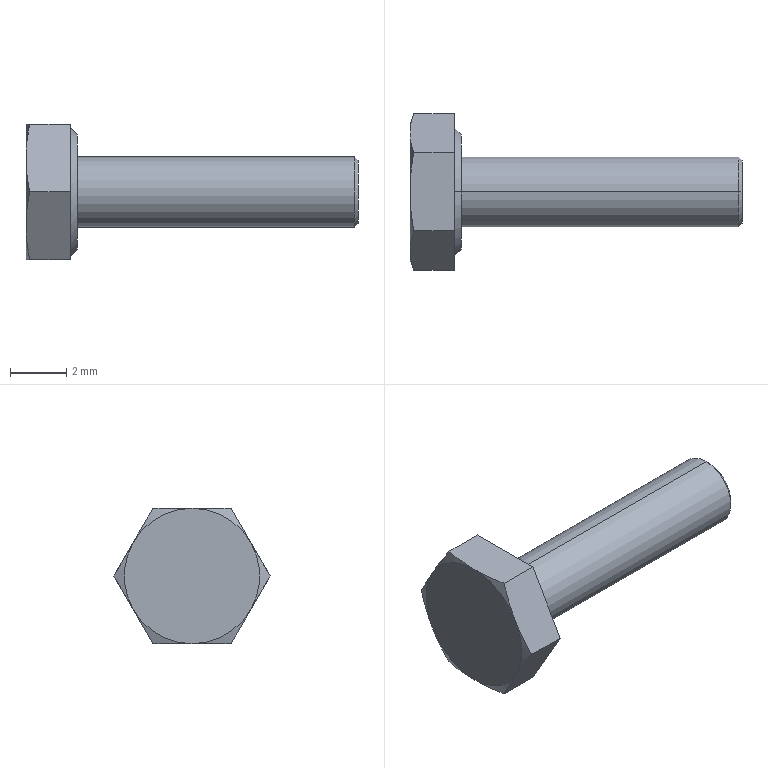Part | SolidWorks | features RevCut 3, Boss 1, Chamfer 1, Extrusion 1, Fillet 1, LPattern 1 | 1 solid | 22 faces | box 11.825 x 5.566 x 4.82 mm | volume 84.307 mm3 | cone 10 | plane 10 | cylinder 2 | commonest cylinder face diameters 2.5 x2
STEP:
#1=CARTESIAN_POINT('',(11.825,0.,-1.125));
#2=VERTEX_POINT('',#1);
#3=CARTESIAN_POINT('',(11.825,0.,1.125));
#4=VERTEX_POINT('',#3);
#5=CARTESIAN_POINT('',(11.825,0.,0.));
#6=DIRECTION('',(1.,0.,0.));
#7=DIRECTION('',(0.,0.,-1.));
#8=AXIS2_PLACEMENT_3D('',#5,#6,#7);
#9=CIRCLE('',#8,1.125);
#10=EDGE_CURVE('',#2,#4,#9,.T.);
#11=ORIENTED_EDGE('',*,*,#10,.F.);
#12=CARTESIAN_POINT('',(11.7,0.,-1.25));
#13=VERTEX_POINT('',#12);
#14=CARTESIAN_POINT('',(11.825,0.,-1.125));
#15=DIRECTION('',(-0.7071,0.,-0.7071));
#16=VECTOR('',#15,1000.);
#17=LINE('',#14,#16);
#18=EDGE_CURVE('',#2,#13,#17,.T.);
#19=ORIENTED_EDGE('',*,*,#18,.T.);
#20=CARTESIAN_POINT('',(11.7,0.,1.25));
#21=VERTEX_POINT('',#20);
#22=CARTESIAN_POINT('',(11.7,0.,0.));
#23=DIRECTION('',(-1.,0.,0.));
#24=DIRECTION('',(0.,0.,-1.));
#25=AXIS2_PLACEMENT_3D('',#22,#23,#24);
#26=CIRCLE('',#25,1.25);
#27=EDGE_CURVE('',#21,#13,#26,.T.);
#28=ORIENTED_EDGE('',*,*,#27,.F.);
#29=CARTESIAN_POINT('',(11.825,0.,1.125));
#30=DIRECTION('',(-0.7071,0.,0.7071));
#31=VECTOR('',#30,1000.);
#32=LINE('',#29,#31);
#33=EDGE_CURVE('',#4,#21,#32,.T.);
#34=ORIENTED_EDGE('',*,*,#33,.F.);
#35=EDGE_LOOP('',(#11,#19,#28,#34));
#36=FACE_OUTER_BOUND('',#35,.T.);
#37=CARTESIAN_POINT('',(11.825,0.,0.));
#38=DIRECTION('',(-1.,0.,0.));
#39=DIRECTION('',(0.,0.,1.));
#40=AXIS2_PLACEMENT_3D('',#37,#38,#39);
#41=CONICAL_SURFACE('',#40,1.125,0.7854);
#42=ADVANCED_FACE('',(#36),#41,.T.);
#43=ORIENTED_EDGE('',*,*,#27,.T.);
#44=CARTESIAN_POINT('',(1.825,0.,-1.25));
#45=VERTEX_POINT('',#44);
#46=CARTESIAN_POINT('',(11.825,0.,-1.25));
#47=DIRECTION('',(-1.,0.,0.));
#48=VECTOR('',#47,1000.);
#49=LINE('',#46,#48);
#50=EDGE_CURVE('',#13,#45,#49,.T.);
#51=ORIENTED_EDGE('',*,*,#50,.T.);
#52=CARTESIAN_POINT('',(1.825,0.,1.25));
#53=VERTEX_POINT('',#52);
#54=CARTESIAN_POINT('',(1.825,0.,0.));
#55=DIRECTION('',(1.,0.,0.));
#56=DIRECTION('',(0.,0.,-1.));
#57=AXIS2_PLACEMENT_3D('',#54,#55,#56);
#58=CIRCLE('',#57,1.25);
#59=EDGE_CURVE('',#45,#53,#58,.T.);
#60=ORIENTED_EDGE('',*,*,#59,.T.);
#61=CARTESIAN_POINT('',(11.825,0.,1.25));
#62=DIRECTION('',(-1.,0.,0.));
#63=VECTOR('',#62,1000.);
#64=LINE('',#61,#63);
#65=EDGE_CURVE('',#21,#53,#64,.T.);
#66=ORIENTED_EDGE('',*,*,#65,.F.);
#67=EDGE_LOOP('',(#43,#51,#60,#66));
#68=FACE_OUTER_BOUND('',#67,.T.);
#69=CARTESIAN_POINT('',(11.825,0.,0.));
#70=DIRECTION('',(-1.,0.,0.));
#71=DIRECTION('',(0.,0.,1.));
#72=AXIS2_PLACEMENT_3D('',#69,#70,#71);
#73=CYLINDRICAL_SURFACE('',#72,1.25);
#74=ADVANCED_FACE('',(#68),#73,.T.);
#75=CARTESIAN_POINT('',(1.825,0.,2.035));
#76=VERTEX_POINT('',#75);
#77=CARTESIAN_POINT('',(1.825,0.,-2.035));
#78=VERTEX_POINT('',#77);
#79=CARTESIAN_POINT('',(1.825,0.,0.));
#80=DIRECTION('',(-1.,0.,0.));
#81=DIRECTION('',(0.,0.,1.));
#82=AXIS2_PLACEMENT_3D('',#79,#80,#81);
#83=CIRCLE('',#82,2.035);
#84=EDGE_CURVE('',#76,#78,#83,.T.);
#85=ORIENTED_EDGE('',*,*,#84,.T.);
#86=CARTESIAN_POINT('',(1.575,0.,-2.285));
#87=VERTEX_POINT('',#86);
#88=CARTESIAN_POINT('',(1.575,0.,-2.285));
#89=DIRECTION('',(-0.7071,0.,-0.7071));
#90=VECTOR('',#89,1000.);
#91=LINE('',#88,#90);
#92=EDGE_CURVE('',#78,#87,#91,.T.);
#93=ORIENTED_EDGE('',*,*,#92,.T.);
#94=CARTESIAN_POINT('',(1.575,0.,2.285));
#95=VERTEX_POINT('',#94);
#96=CARTESIAN_POINT('',(1.575,0.,0.));
#97=DIRECTION('',(-1.,0.,0.));
#98=DIRECTION('',(0.,0.,1.));
#99=AXIS2_PLACEMENT_3D('',#96,#97,#98);
#100=CIRCLE('',#99,2.285);
#101=EDGE_CURVE('',#95,#87,#100,.T.);
#102=ORIENTED_EDGE('',*,*,#101,.F.);
#103=CARTESIAN_POINT('',(1.575,0.,2.285));
#104=DIRECTION('',(-0.7071,0.,0.7071));
#105=VECTOR('',#104,1000.);
#106=LINE('',#103,#105);
#107=EDGE_CURVE('',#76,#95,#106,.T.);
#108=ORIENTED_EDGE('',*,*,#107,.F.);
#109=EDGE_LOOP('',(#85,#93,#102,#108));
#110=FACE_OUTER_BOUND('',#109,.T.);
#111=CARTESIAN_POINT('',(1.575,0.,0.));
#112=DIRECTION('',(-1.,0.,0.));
#113=DIRECTION('',(0.,0.,1.));
#114=AXIS2_PLACEMENT_3D('',#111,#112,#113);
#115=CONICAL_SURFACE('',#114,2.285,0.7854);
#116=ADVANCED_FACE('',(#110),#115,.T.);
#117=ORIENTED_EDGE('',*,*,#84,.F.);
#118=CARTESIAN_POINT('',(1.825,0.,0.));
#119=DIRECTION('',(-1.,0.,0.));
#120=DIRECTION('',(0.,0.,1.));
#121=AXIS2_PLACEMENT_3D('',#118,#119,#120);
#122=CIRCLE('',#121,2.035);
#123=EDGE_CURVE('',#78,#76,#122,.T.);
#124=ORIENTED_EDGE('',*,*,#123,.F.);
#125=EDGE_LOOP('',(#117,#124));
#126=FACE_OUTER_BOUND('',#125,.T.);
#127=CARTESIAN_POINT('',(1.825,0.,0.));
#128=DIRECTION('',(1.,0.,0.));
#129=DIRECTION('',(0.,0.,-1.));
#130=AXIS2_PLACEMENT_3D('',#127,#128,#129);
#131=CIRCLE('',#130,1.25);
#132=EDGE_CURVE('',#53,#45,#131,.T.);
#133=ORIENTED_EDGE('',*,*,#132,.F.);
#134=ORIENTED_EDGE('',*,*,#59,.F.);
#135=EDGE_LOOP('',(#133,#134));
#136=FACE_BOUND('',#135,.T.);
#137=CARTESIAN_POINT('',(1.825,-1.391,-2.41));
#138=DIRECTION('',(1.,0.,0.));
#139=DIRECTION('',(0.,0.,-1.));
#140=AXIS2_PLACEMENT_3D('',#137,#138,#139);
#141=PLANE('',#140);
#142=ADVANCED_FACE('',(#126,#136),#141,.T.);
#143=CARTESIAN_POINT('',(0.1357,-1.391,-2.41));
#144=VERTEX_POINT('',#143);
#145=CARTESIAN_POINT('',(0.,-2.087,-1.205));
#146=VERTEX_POINT('',#145);
#147=CARTESIAN_POINT('',(0.1357,-1.391,-2.41));
#148=CARTESIAN_POINT('',(0.05129,-1.623,-2.008));
#149=CARTESIAN_POINT('',(0.,-1.855,-1.607));
#150=CARTESIAN_POINT('',(0.,-2.087,-1.205));
#151=B_SPLINE_CURVE_WITH_KNOTS('',3,(#147,#148,#149,#150),.UNSPECIFIED.,.F.,.F.,(4,4),(0.000000231,0.001392),.UNSPECIFIED.);
#152=EDGE_CURVE('',#144,#146,#151,.T.);
#153=ORIENTED_EDGE('',*,*,#152,.F.);
#154=CARTESIAN_POINT('',(1.575,-1.391,-2.41));
#155=VERTEX_POINT('',#154);
#156=CARTESIAN_POINT('',(1.825,-1.391,-2.41));
#157=DIRECTION('',(-1.,0.,0.));
#158=VECTOR('',#157,1000.);
#159=LINE('',#156,#158);
#160=EDGE_CURVE('',#155,#144,#159,.T.);
#161=ORIENTED_EDGE('',*,*,#160,.F.);
#162=CARTESIAN_POINT('',(1.575,-2.783,0.));
#163=VERTEX_POINT('',#162);
#164=CARTESIAN_POINT('',(1.575,-2.783,0.));
#165=DIRECTION('',(0.,0.5,-0.866));
#166=VECTOR('',#165,1000.);
#167=LINE('',#164,#166);
#168=EDGE_CURVE('',#163,#155,#167,.T.);
#169=ORIENTED_EDGE('',*,*,#168,.F.);
#170=CARTESIAN_POINT('',(0.1357,-2.783,0.));
#171=VERTEX_POINT('',#170);
#172=CARTESIAN_POINT('',(1.825,-2.783,0.));
#173=DIRECTION('',(-1.,0.,0.));
#174=VECTOR('',#173,1000.);
#175=LINE('',#172,#174);
#176=EDGE_CURVE('',#163,#171,#175,.T.);
#177=ORIENTED_EDGE('',*,*,#176,.T.);
#178=CARTESIAN_POINT('',(0.,-2.087,-1.205));
#179=CARTESIAN_POINT('',(0.,-2.319,-0.8033));
#180=CARTESIAN_POINT('',(0.05129,-2.551,-0.4017));
#181=CARTESIAN_POINT('',(0.1357,-2.783,0.));
#182=B_SPLINE_CURVE_WITH_KNOTS('',3,(#178,#179,#180,#181),.UNSPECIFIED.,.F.,.F.,(4,4),(0.001392,0.002783),.UNSPECIFIED.);
#183=EDGE_CURVE('',#146,#171,#182,.T.);
#184=ORIENTED_EDGE('',*,*,#183,.F.);
#185=EDGE_LOOP('',(#153,#161,#169,#177,#184));
#186=FACE_OUTER_BOUND('',#185,.T.);
#187=CARTESIAN_POINT('',(1.825,-2.783,0.));
#188=DIRECTION('',(0.,0.866,0.5));
#189=DIRECTION('',(0.,-0.5,0.866));
#190=AXIS2_PLACEMENT_3D('',#187,#188,#189);
#191=PLANE('',#190);
#192=ADVANCED_FACE('',(#186),#191,.F.);
#193=CARTESIAN_POINT('',(0.1357,1.391,-2.41));
#194=VERTEX_POINT('',#193);
#195=CARTESIAN_POINT('',(0.,0.,-2.41));
#196=VERTEX_POINT('',#195);
#197=CARTESIAN_POINT('',(0.1357,1.391,-2.41));
#198=CARTESIAN_POINT('',(0.05152,0.9289,-2.41));
#199=CARTESIAN_POINT('',(0.,0.4648,-2.41));
#200=CARTESIAN_POINT('',(0.,0.,-2.41));
#201=B_SPLINE_CURVE_WITH_KNOTS('',3,(#197,#198,#199,#200),.UNSPECIFIED.,.F.,.F.,(4,4),(0.005017,0.00642),.UNSPECIFIED.);
#202=EDGE_CURVE('',#194,#196,#201,.T.);
#203=ORIENTED_EDGE('',*,*,#202,.F.);
#204=CARTESIAN_POINT('',(1.575,1.391,-2.41));
#205=VERTEX_POINT('',#204);
#206=CARTESIAN_POINT('',(1.825,1.391,-2.41));
#207=DIRECTION('',(-1.,0.,0.));
#208=VECTOR('',#207,1000.);
#209=LINE('',#206,#208);
#210=EDGE_CURVE('',#205,#194,#209,.T.);
#211=ORIENTED_EDGE('',*,*,#210,.F.);
#212=CARTESIAN_POINT('',(1.575,-1.391,-2.41));
#213=DIRECTION('',(0.,1.,0.));
#214=VECTOR('',#213,1000.);
#215=LINE('',#212,#214);
#216=EDGE_CURVE('',#155,#205,#215,.T.);
#217=ORIENTED_EDGE('',*,*,#216,.F.);
#218=ORIENTED_EDGE('',*,*,#160,.T.);
#219=CARTESIAN_POINT('',(0.,0.,-2.41));
#220=CARTESIAN_POINT('',(0.,-0.4634,-2.41));
#221=CARTESIAN_POINT('',(0.05185,-0.9307,-2.41));
#222=CARTESIAN_POINT('',(0.1357,-1.391,-2.41));
#223=B_SPLINE_CURVE_WITH_KNOTS('',3,(#219,#220,#221,#222),.UNSPECIFIED.,.F.,.F.,(4,4),(0.00642,0.007819),.UNSPECIFIED.);
#224=EDGE_CURVE('',#196,#144,#223,.T.);
#225=ORIENTED_EDGE('',*,*,#224,.F.);
#226=EDGE_LOOP('',(#203,#211,#217,#218,#225));
#227=FACE_OUTER_BOUND('',#226,.T.);
#228=CARTESIAN_POINT('',(1.825,-1.391,-2.41));
#229=DIRECTION('',(0.,0.,1.));
#230=DIRECTION('',(1.,0.,0.));
#231=AXIS2_PLACEMENT_3D('',#228,#229,#230);
#232=PLANE('',#231);
#233=ADVANCED_FACE('',(#227),#232,.F.);
#234=CARTESIAN_POINT('',(0.1357,2.783,0.));
#235=VERTEX_POINT('',#234);
#236=CARTESIAN_POINT('',(0.,2.087,-1.205));
#237=VERTEX_POINT('',#236);
#238=CARTESIAN_POINT('',(0.1357,2.783,0.));
#239=CARTESIAN_POINT('',(0.05129,2.551,-0.4017));
#240=CARTESIAN_POINT('',(0.,2.319,-0.8033));
#241=CARTESIAN_POINT('',(0.,2.087,-1.205));
#242=B_SPLINE_CURVE_WITH_KNOTS('',3,(#238,#239,#240,#241),.UNSPECIFIED.,.F.,.F.,(4,4),(0.000000231,0.001392),.UNSPECIFIED.);
#243=EDGE_CURVE('',#235,#237,#242,.T.);
#244=ORIENTED_EDGE('',*,*,#243,.F.);
#245=CARTESIAN_POINT('',(1.575,2.783,0.));
#246=VERTEX_POINT('',#245);
#247=CARTESIAN_POINT('',(1.825,2.783,0.));
#248=DIRECTION('',(-1.,0.,0.));
#249=VECTOR('',#248,1000.);
#250=LINE('',#247,#249);
#251=EDGE_CURVE('',#246,#235,#250,.T.);
#252=ORIENTED_EDGE('',*,*,#251,.F.);
#253=CARTESIAN_POINT('',(1.575,1.391,-2.41));
#254=DIRECTION('',(0.,0.5,0.866));
#255=VECTOR('',#254,1000.);
#256=LINE('',#253,#255);
#257=EDGE_CURVE('',#205,#246,#256,.T.);
#258=ORIENTED_EDGE('',*,*,#257,.F.);
#259=ORIENTED_EDGE('',*,*,#210,.T.);
#260=CARTESIAN_POINT('',(0.,2.087,-1.205));
#261=CARTESIAN_POINT('',(0.,1.855,-1.607));
#262=CARTESIAN_POINT('',(0.05129,1.623,-2.008));
#263=CARTESIAN_POINT('',(0.1357,1.391,-2.41));
#264=B_SPLINE_CURVE_WITH_KNOTS('',3,(#260,#261,#262,#263),.UNSPECIFIED.,.F.,.F.,(4,4),(0.001392,0.002783),.UNSPECIFIED.);
#265=EDGE_CURVE('',#237,#194,#264,.T.);
#266=ORIENTED_EDGE('',*,*,#265,.F.);
#267=EDGE_LOOP('',(#244,#252,#258,#259,#266));
#268=FACE_OUTER_BOUND('',#267,.T.);
#269=CARTESIAN_POINT('',(1.825,1.391,-2.41));
#270=DIRECTION('',(0.,-0.866,0.5));
#271=DIRECTION('',(0.,-0.5,-0.866));
#272=AXIS2_PLACEMENT_3D('',#269,#270,#271);
#273=PLANE('',#272);
#274=ADVANCED_FACE('',(#268),#273,.F.);
#275=CARTESIAN_POINT('',(0.1357,1.391,2.41));
#276=VERTEX_POINT('',#275);
#277=CARTESIAN_POINT('',(0.,2.087,1.205));
#278=VERTEX_POINT('',#277);
#279=CARTESIAN_POINT('',(0.1357,1.391,2.41));
#280=CARTESIAN_POINT('',(0.05129,1.623,2.008));
#281=CARTESIAN_POINT('',(0.,1.855,1.607));
#282=CARTESIAN_POINT('',(0.,2.087,1.205));
#283=B_SPLINE_CURVE_WITH_KNOTS('',3,(#279,#280,#281,#282),.UNSPECIFIED.,.F.,.F.,(4,4),(0.000000231,0.001392),.UNSPECIFIED.);
#284=EDGE_CURVE('',#276,#278,#283,.T.);
#285=ORIENTED_EDGE('',*,*,#284,.F.);
#286=CARTESIAN_POINT('',(1.575,1.391,2.41));
#287=VERTEX_POINT('',#286);
#288=CARTESIAN_POINT('',(1.825,1.391,2.41));
#289=DIRECTION('',(-1.,0.,0.));
#290=VECTOR('',#289,1000.);
#291=LINE('',#288,#290);
#292=EDGE_CURVE('',#287,#276,#291,.T.);
#293=ORIENTED_EDGE('',*,*,#292,.F.);
#294=CARTESIAN_POINT('',(1.575,2.783,0.));
#295=DIRECTION('',(0.,-0.5,0.866));
#296=VECTOR('',#295,1000.);
#297=LINE('',#294,#296);
#298=EDGE_CURVE('',#246,#287,#297,.T.);
#299=ORIENTED_EDGE('',*,*,#298,.F.);
#300=ORIENTED_EDGE('',*,*,#251,.T.);
#301=CARTESIAN_POINT('',(0.,2.087,1.205));
#302=CARTESIAN_POINT('',(0.,2.319,0.8033));
#303=CARTESIAN_POINT('',(0.05129,2.551,0.4017));
#304=CARTESIAN_POINT('',(0.1357,2.783,0.));
#305=B_SPLINE_CURVE_WITH_KNOTS('',3,(#301,#302,#303,#304),.UNSPECIFIED.,.F.,.F.,(4,4),(0.001392,0.002783),.UNSPECIFIED.);
#306=EDGE_CURVE('',#278,#235,#305,.T.);
#307=ORIENTED_EDGE('',*,*,#306,.F.);
#308=EDGE_LOOP('',(#285,#293,#299,#300,#307));
#309=FACE_OUTER_BOUND('',#308,.T.);
#310=CARTESIAN_POINT('',(1.825,2.783,0.));
#311=DIRECTION('',(0.,-0.866,-0.5));
#312=DIRECTION('',(0.,0.5,-0.866));
#313=AXIS2_PLACEMENT_3D('',#310,#311,#312);
#314=PLANE('',#313);
#315=ADVANCED_FACE('',(#309),#314,.F.);
#316=CARTESIAN_POINT('',(0.1357,-1.391,2.41));
#317=VERTEX_POINT('',#316);
#318=CARTESIAN_POINT('',(0.,0.,2.41));
#319=VERTEX_POINT('',#318);
#320=CARTESIAN_POINT('',(0.1357,-1.391,2.41));
#321=CARTESIAN_POINT('',(0.05185,-0.9307,2.41));
#322=CARTESIAN_POINT('',(0.,-0.4634,2.41));
#323=CARTESIAN_POINT('',(0.,0.,2.41));
#324=B_SPLINE_CURVE_WITH_KNOTS('',3,(#320,#321,#322,#323),.UNSPECIFIED.,.F.,.F.,(4,4),(0.002367,0.003769),.UNSPECIFIED.);
#325=EDGE_CURVE('',#317,#319,#324,.T.);
#326=ORIENTED_EDGE('',*,*,#325,.F.);
#327=CARTESIAN_POINT('',(1.575,-1.391,2.41));
#328=VERTEX_POINT('',#327);
#329=CARTESIAN_POINT('',(1.825,-1.391,2.41));
#330=DIRECTION('',(-1.,0.,0.));
#331=VECTOR('',#330,1000.);
#332=LINE('',#329,#331);
#333=EDGE_CURVE('',#328,#317,#332,.T.);
#334=ORIENTED_EDGE('',*,*,#333,.F.);
#335=CARTESIAN_POINT('',(1.575,1.391,2.41));
#336=DIRECTION('',(0.,-1.,0.));
#337=VECTOR('',#336,1000.);
#338=LINE('',#335,#337);
#339=EDGE_CURVE('',#287,#328,#338,.T.);
#340=ORIENTED_EDGE('',*,*,#339,.F.);
#341=ORIENTED_EDGE('',*,*,#292,.T.);
#342=CARTESIAN_POINT('',(0.,0.,2.41));
#343=CARTESIAN_POINT('',(0.,0.4648,2.41));
#344=CARTESIAN_POINT('',(0.05152,0.9289,2.41));
#345=CARTESIAN_POINT('',(0.1357,1.391,2.41));
#346=B_SPLINE_CURVE_WITH_KNOTS('',3,(#342,#343,#344,#345),.UNSPECIFIED.,.F.,.F.,(4,4),(0.003769,0.005176),.UNSPECIFIED.);
#347=EDGE_CURVE('',#319,#276,#346,.T.);
#348=ORIENTED_EDGE('',*,*,#347,.F.);
#349=EDGE_LOOP('',(#326,#334,#340,#341,#348));
#350=FACE_OUTER_BOUND('',#349,.T.);
#351=CARTESIAN_POINT('',(1.825,1.391,2.41));
#352=DIRECTION('',(0.,0.,-1.));
#353=DIRECTION('',(0.,1.,0.));
#354=AXIS2_PLACEMENT_3D('',#351,#352,#353);
#355=PLANE('',#354);
#356=ADVANCED_FACE('',(#350),#355,.F.);
#357=CARTESIAN_POINT('',(0.,-2.087,1.205));
#358=VERTEX_POINT('',#357);
#359=CARTESIAN_POINT('',(0.1357,-2.783,0.));
#360=CARTESIAN_POINT('',(0.05129,-2.551,0.4017));
#361=CARTESIAN_POINT('',(0.,-2.319,0.8033));
#362=CARTESIAN_POINT('',(0.,-2.087,1.205));
#363=B_SPLINE_CURVE_WITH_KNOTS('',3,(#359,#360,#361,#362),.UNSPECIFIED.,.F.,.F.,(4,4),(0.000000231,0.001392),.UNSPECIFIED.);
#364=EDGE_CURVE('',#171,#358,#363,.T.);
#365=ORIENTED_EDGE('',*,*,#364,.F.);
#366=ORIENTED_EDGE('',*,*,#176,.F.);
#367=CARTESIAN_POINT('',(1.575,-1.391,2.41));
#368=DIRECTION('',(0.,-0.5,-0.866));
#369=VECTOR('',#368,1000.);
#370=LINE('',#367,#369);
#371=EDGE_CURVE('',#328,#163,#370,.T.);
#372=ORIENTED_EDGE('',*,*,#371,.F.);
#373=ORIENTED_EDGE('',*,*,#333,.T.);
#374=CARTESIAN_POINT('',(0.,-2.087,1.205));
#375=CARTESIAN_POINT('',(0.,-1.855,1.607));
#376=CARTESIAN_POINT('',(0.05129,-1.623,2.008));
#377=CARTESIAN_POINT('',(0.1357,-1.391,2.41));
#378=B_SPLINE_CURVE_WITH_KNOTS('',3,(#374,#375,#376,#377),.UNSPECIFIED.,.F.,.F.,(4,4),(0.001392,0.002783),.UNSPECIFIED.);
#379=EDGE_CURVE('',#358,#317,#378,.T.);
#380=ORIENTED_EDGE('',*,*,#379,.F.);
#381=EDGE_LOOP('',(#365,#366,#372,#373,#380));
#382=FACE_OUTER_BOUND('',#381,.T.);
#383=CARTESIAN_POINT('',(1.825,-1.391,2.41));
#384=DIRECTION('',(0.,0.866,-0.5));
#385=DIRECTION('',(0.,0.5,0.866));
#386=AXIS2_PLACEMENT_3D('',#383,#384,#385);
#387=PLANE('',#386);
#388=ADVANCED_FACE('',(#382),#387,.F.);
#389=ORIENTED_EDGE('',*,*,#101,.T.);
#390=CARTESIAN_POINT('',(1.575,0.,0.));
#391=DIRECTION('',(-1.,0.,0.));
#392=DIRECTION('',(0.,0.,1.));
#393=AXIS2_PLACEMENT_3D('',#390,#391,#392);
#394=CIRCLE('',#393,2.285);
#395=EDGE_CURVE('',#87,#95,#394,.T.);
#396=ORIENTED_EDGE('',*,*,#395,.T.);
#397=EDGE_LOOP('',(#389,#396));
#398=FACE_BOUND('',#397,.T.);
#399=ORIENTED_EDGE('',*,*,#168,.T.);
#400=ORIENTED_EDGE('',*,*,#216,.T.);
#401=ORIENTED_EDGE('',*,*,#257,.T.);
#402=ORIENTED_EDGE('',*,*,#298,.T.);
#403=ORIENTED_EDGE('',*,*,#339,.T.);
#404=ORIENTED_EDGE('',*,*,#371,.T.);
#405=EDGE_LOOP('',(#399,#400,#401,#402,#403,#404));
#406=FACE_OUTER_BOUND('',#405,.T.);
#407=CARTESIAN_POINT('',(1.575,2.285,0.));
#408=DIRECTION('',(1.,0.,0.));
#409=DIRECTION('',(0.,0.,-1.));
#410=AXIS2_PLACEMENT_3D('',#407,#408,#409);
#411=PLANE('',#410);
#412=ADVANCED_FACE('',(#398,#406),#411,.T.);
#413=ORIENTED_EDGE('',*,*,#92,.F.);
#414=ORIENTED_EDGE('',*,*,#123,.T.);
#415=ORIENTED_EDGE('',*,*,#107,.T.);
#416=ORIENTED_EDGE('',*,*,#395,.F.);
#417=EDGE_LOOP('',(#413,#414,#415,#416));
#418=FACE_OUTER_BOUND('',#417,.T.);
#419=CARTESIAN_POINT('',(1.575,0.,0.));
#420=DIRECTION('',(-1.,0.,0.));
#421=DIRECTION('',(0.,0.,1.));
#422=AXIS2_PLACEMENT_3D('',#419,#420,#421);
#423=CONICAL_SURFACE('',#422,2.285,0.7854);
#424=ADVANCED_FACE('',(#418),#423,.T.);
#425=ORIENTED_EDGE('',*,*,#224,.T.);
#426=ORIENTED_EDGE('',*,*,#152,.T.);
#427=CARTESIAN_POINT('',(0.,0.,0.));
#428=DIRECTION('',(1.,0.,0.));
#429=DIRECTION('',(0.,0.,-1.));
#430=AXIS2_PLACEMENT_3D('',#427,#428,#429);
#431=CIRCLE('',#430,2.41);
#432=EDGE_CURVE('',#146,#196,#431,.T.);
#433=ORIENTED_EDGE('',*,*,#432,.T.);
#434=EDGE_LOOP('',(#425,#426,#433));
#435=FACE_OUTER_BOUND('',#434,.T.);
#436=CARTESIAN_POINT('',(0.,0.,0.));
#437=DIRECTION('',(1.,0.,0.));
#438=DIRECTION('',(0.,0.,-1.));
#439=AXIS2_PLACEMENT_3D('',#436,#437,#438);
#440=CONICAL_SURFACE('',#439,2.41,1.222);
#441=ADVANCED_FACE('',(#435),#440,.T.);
#442=ORIENTED_EDGE('',*,*,#183,.T.);
#443=ORIENTED_EDGE('',*,*,#364,.T.);
#444=CARTESIAN_POINT('',(0.,0.,0.));
#445=DIRECTION('',(1.,0.,0.));
#446=DIRECTION('',(0.,0.,-1.));
#447=AXIS2_PLACEMENT_3D('',#444,#445,#446);
#448=CIRCLE('',#447,2.41);
#449=EDGE_CURVE('',#358,#146,#448,.T.);
#450=ORIENTED_EDGE('',*,*,#449,.T.);
#451=EDGE_LOOP('',(#442,#443,#450));
#452=FACE_OUTER_BOUND('',#451,.T.);
#453=CARTESIAN_POINT('',(0.,0.,0.));
#454=DIRECTION('',(1.,0.,0.));
#455=DIRECTION('',(0.,0.,-1.));
#456=AXIS2_PLACEMENT_3D('',#453,#454,#455);
#457=CONICAL_SURFACE('',#456,2.41,1.222);
#458=ADVANCED_FACE('',(#452),#457,.T.);
#459=ORIENTED_EDGE('',*,*,#325,.T.);
#460=CARTESIAN_POINT('',(0.,0.,0.));
#461=DIRECTION('',(1.,0.,0.));
#462=DIRECTION('',(0.,0.,-1.));
#463=AXIS2_PLACEMENT_3D('',#460,#461,#462);
#464=CIRCLE('',#463,2.41);
#465=EDGE_CURVE('',#319,#358,#464,.T.);
#466=ORIENTED_EDGE('',*,*,#465,.T.);
#467=ORIENTED_EDGE('',*,*,#379,.T.);
#468=EDGE_LOOP('',(#459,#466,#467));
#469=FACE_OUTER_BOUND('',#468,.T.);
#470=CARTESIAN_POINT('',(0.,0.,0.));
#471=DIRECTION('',(1.,0.,0.));
#472=DIRECTION('',(0.,0.,-1.));
#473=AXIS2_PLACEMENT_3D('',#470,#471,#472);
#474=CONICAL_SURFACE('',#473,2.41,1.222);
#475=ADVANCED_FACE('',(#469),#474,.T.);
#476=ORIENTED_EDGE('',*,*,#284,.T.);
#477=CARTESIAN_POINT('',(0.,0.,0.));
#478=DIRECTION('',(-1.,0.,0.));
#479=DIRECTION('',(0.,0.,1.));
#480=AXIS2_PLACEMENT_3D('',#477,#478,#479);
#481=CIRCLE('',#480,2.41);
#482=EDGE_CURVE('',#319,#278,#481,.T.);
#483=ORIENTED_EDGE('',*,*,#482,.F.);
#484=ORIENTED_EDGE('',*,*,#347,.T.);
#485=EDGE_LOOP('',(#476,#483,#484));
#486=FACE_OUTER_BOUND('',#485,.T.);
#487=CARTESIAN_POINT('',(0.,0.,0.));
#488=DIRECTION('',(1.,0.,0.));
#489=DIRECTION('',(0.,0.,-1.));
#490=AXIS2_PLACEMENT_3D('',#487,#488,#489);
#491=CONICAL_SURFACE('',#490,2.41,1.222);
#492=ADVANCED_FACE('',(#486),#491,.T.);
#493=ORIENTED_EDGE('',*,*,#243,.T.);
#494=CARTESIAN_POINT('',(0.,0.,0.));
#495=DIRECTION('',(1.,0.,0.));
#496=DIRECTION('',(0.,0.,-1.));
#497=AXIS2_PLACEMENT_3D('',#494,#495,#496);
#498=CIRCLE('',#497,2.41);
#499=EDGE_CURVE('',#237,#278,#498,.T.);
#500=ORIENTED_EDGE('',*,*,#499,.T.);
#501=ORIENTED_EDGE('',*,*,#306,.T.);
#502=EDGE_LOOP('',(#493,#500,#501));
#503=FACE_OUTER_BOUND('',#502,.T.);
#504=CARTESIAN_POINT('',(0.,0.,0.));
#505=DIRECTION('',(1.,0.,0.));
#506=DIRECTION('',(0.,0.,-1.));
#507=AXIS2_PLACEMENT_3D('',#504,#505,#506);
#508=CONICAL_SURFACE('',#507,2.41,1.222);
#509=ADVANCED_FACE('',(#503),#508,.T.);
#510=ORIENTED_EDGE('',*,*,#265,.T.);
#511=ORIENTED_EDGE('',*,*,#202,.T.);
#512=CARTESIAN_POINT('',(0.,0.,0.));
#513=DIRECTION('',(1.,0.,0.));
#514=DIRECTION('',(0.,0.,-1.));
#515=AXIS2_PLACEMENT_3D('',#512,#513,#514);
#516=CIRCLE('',#515,2.41);
#517=EDGE_CURVE('',#196,#237,#516,.T.);
#518=ORIENTED_EDGE('',*,*,#517,.T.);
#519=EDGE_LOOP('',(#510,#511,#518));
#520=FACE_OUTER_BOUND('',#519,.T.);
#521=CARTESIAN_POINT('',(0.,0.,0.));
#522=DIRECTION('',(1.,0.,0.));
#523=DIRECTION('',(0.,0.,-1.));
#524=AXIS2_PLACEMENT_3D('',#521,#522,#523);
#525=CONICAL_SURFACE('',#524,2.41,1.222);
#526=ADVANCED_FACE('',(#520),#525,.T.);
#527=ORIENTED_EDGE('',*,*,#517,.F.);
#528=ORIENTED_EDGE('',*,*,#432,.F.);
#529=ORIENTED_EDGE('',*,*,#449,.F.);
#530=ORIENTED_EDGE('',*,*,#465,.F.);
#531=ORIENTED_EDGE('',*,*,#482,.T.);
#532=ORIENTED_EDGE('',*,*,#499,.F.);
#533=EDGE_LOOP('',(#527,#528,#529,#530,#531,#532));
#534=FACE_OUTER_BOUND('',#533,.T.);
#535=CARTESIAN_POINT('',(0.,-1.391,-2.41));
#536=DIRECTION('',(1.,0.,0.));
#537=DIRECTION('',(0.,0.,-1.));
#538=AXIS2_PLACEMENT_3D('',#535,#536,#537);
#539=PLANE('',#538);
#540=ADVANCED_FACE('',(#534),#539,.F.);
#541=ORIENTED_EDGE('',*,*,#50,.F.);
#542=CARTESIAN_POINT('',(11.7,0.,0.));
#543=DIRECTION('',(-1.,0.,0.));
#544=DIRECTION('',(0.,0.,-1.));
#545=AXIS2_PLACEMENT_3D('',#542,#543,#544);
#546=CIRCLE('',#545,1.25);
#547=EDGE_CURVE('',#13,#21,#546,.T.);
#548=ORIENTED_EDGE('',*,*,#547,.T.);
#549=ORIENTED_EDGE('',*,*,#65,.T.);
#550=ORIENTED_EDGE('',*,*,#132,.T.);
#551=EDGE_LOOP('',(#541,#548,#549,#550));
#552=FACE_OUTER_BOUND('',#551,.T.);
#553=CARTESIAN_POINT('',(11.825,0.,0.));
#554=DIRECTION('',(-1.,0.,0.));
#555=DIRECTION('',(0.,0.,1.));
#556=AXIS2_PLACEMENT_3D('',#553,#554,#555);
#557=CYLINDRICAL_SURFACE('',#556,1.25);
#558=ADVANCED_FACE('',(#552),#557,.T.);
#559=CARTESIAN_POINT('',(11.825,0.,0.));
#560=DIRECTION('',(1.,0.,0.));
#561=DIRECTION('',(0.,0.,-1.));
#562=AXIS2_PLACEMENT_3D('',#559,#560,#561);
#563=CIRCLE('',#562,1.125);
#564=EDGE_CURVE('',#4,#2,#563,.T.);
#565=ORIENTED_EDGE('',*,*,#564,.T.);
#566=ORIENTED_EDGE('',*,*,#10,.T.);
#567=EDGE_LOOP('',(#565,#566));
#568=FACE_OUTER_BOUND('',#567,.T.);
#569=CARTESIAN_POINT('',(11.825,0.,0.));
#570=DIRECTION('',(1.,0.,0.));
#571=DIRECTION('',(0.,0.,-1.));
#572=AXIS2_PLACEMENT_3D('',#569,#570,#571);
#573=PLANE('',#572);
#574=ADVANCED_FACE('',(#568),#573,.T.);
#575=ORIENTED_EDGE('',*,*,#18,.F.);
#576=ORIENTED_EDGE('',*,*,#564,.F.);
#577=ORIENTED_EDGE('',*,*,#33,.T.);
#578=ORIENTED_EDGE('',*,*,#547,.F.);
#579=EDGE_LOOP('',(#575,#576,#577,#578));
#580=FACE_OUTER_BOUND('',#579,.T.);
#581=CARTESIAN_POINT('',(11.825,0.,0.));
#582=DIRECTION('',(-1.,0.,0.));
#583=DIRECTION('',(0.,0.,1.));
#584=AXIS2_PLACEMENT_3D('',#581,#582,#583);
#585=CONICAL_SURFACE('',#584,1.125,0.7854);
#586=ADVANCED_FACE('',(#580),#585,.T.);
#587=CLOSED_SHELL('',(#42,#74,#116,#142,#192,#233,#274,#315,#356,#388,#412,#424,#441,#458,#475,#492,#509,#526,#540,#558,#574,#586));
#588=MANIFOLD_SOLID_BREP('',#587);
#589=CARTESIAN_POINT('',(0.,0.,0.));
#590=DIRECTION('',(0.,0.,1.));
#591=DIRECTION('',(1.,0.,0.));
#592=AXIS2_PLACEMENT_3D('',#589,#590,#591);
#593=(LENGTH_UNIT()NAMED_UNIT(*)SI_UNIT(.MILLI.,.METRE.));
#594=UNCERTAINTY_MEASURE_WITH_UNIT(LENGTH_MEASURE(0.00001),#593,'','');
#595=(NAMED_UNIT(*)PLANE_ANGLE_UNIT()SI_UNIT($,.RADIAN.));
#596=(NAMED_UNIT(*)SI_UNIT($,.STERADIAN.)SOLID_ANGLE_UNIT());
#597=(GEOMETRIC_REPRESENTATION_CONTEXT(3)GLOBAL_UNCERTAINTY_ASSIGNED_CONTEXT((#594))GLOBAL_UNIT_ASSIGNED_CONTEXT((#593,#595,#596))REPRESENTATION_CONTEXT('',''));
#598=ADVANCED_BREP_SHAPE_REPRESENTATION('',(#588,#592),#597);